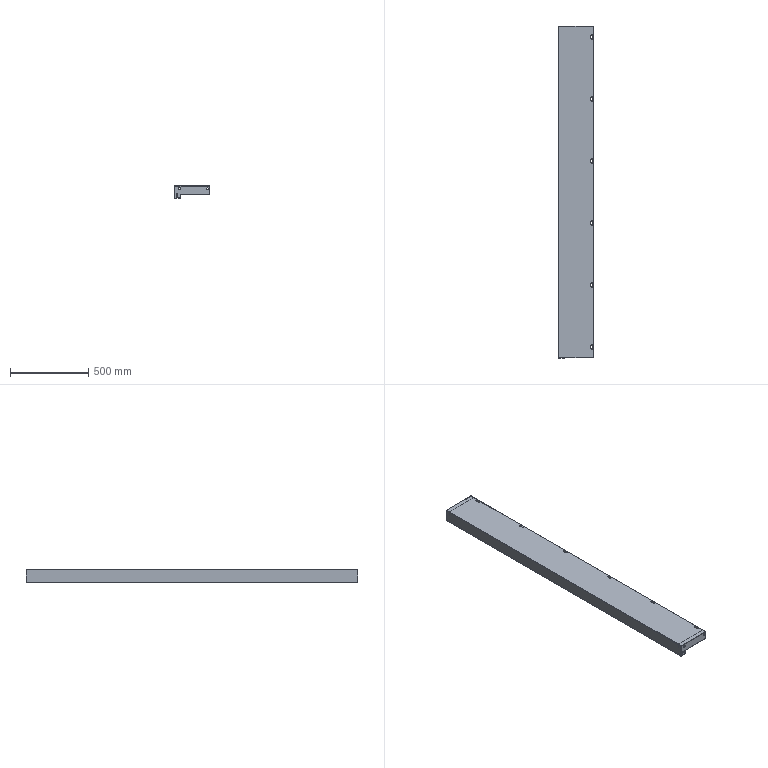Part | SolidWorks | features MirrorCompFeat 1, ReferencePattern 1 | 3 solids | 206 faces | box 225 x 2116 x 80 mm | volume 1110197 mm3 | plane 126 | cylinder 80 | commonest cylinder face diameters 6.2 x28 9 x18 11 x10 3.4 x9 10 x6 1 x5